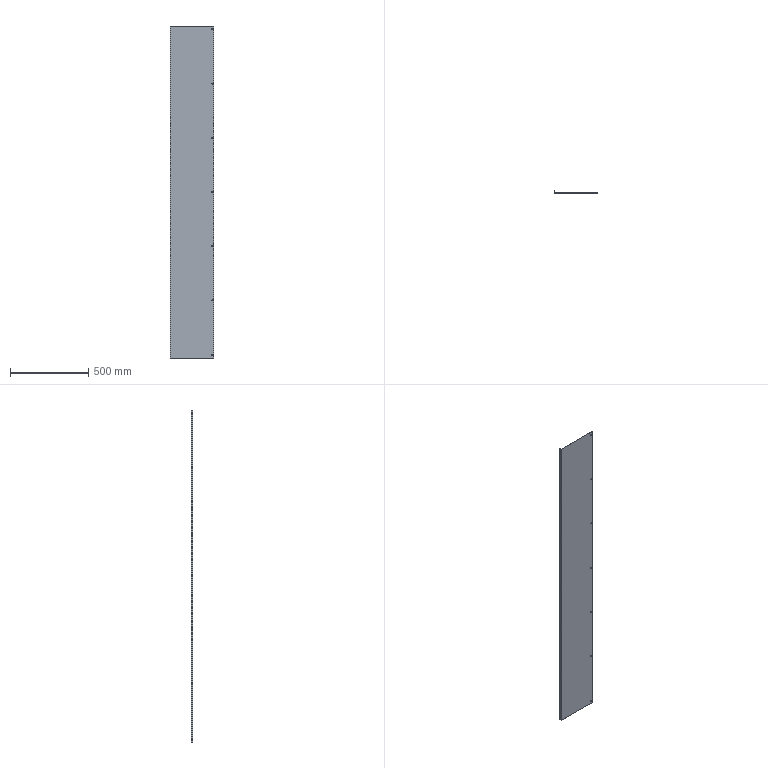Part | SolidWorks | features ICE 4, FlatPattern 1, SMBaseFlange 1, SheetMetal 1 | 1 solid | 77 faces | box 278 x 12 x 2116 mm | volume 610438 mm3 | plane 40 | cylinder 37 | commonest cylinder face diameters 5 x35 0.4 x1 2.4 x1